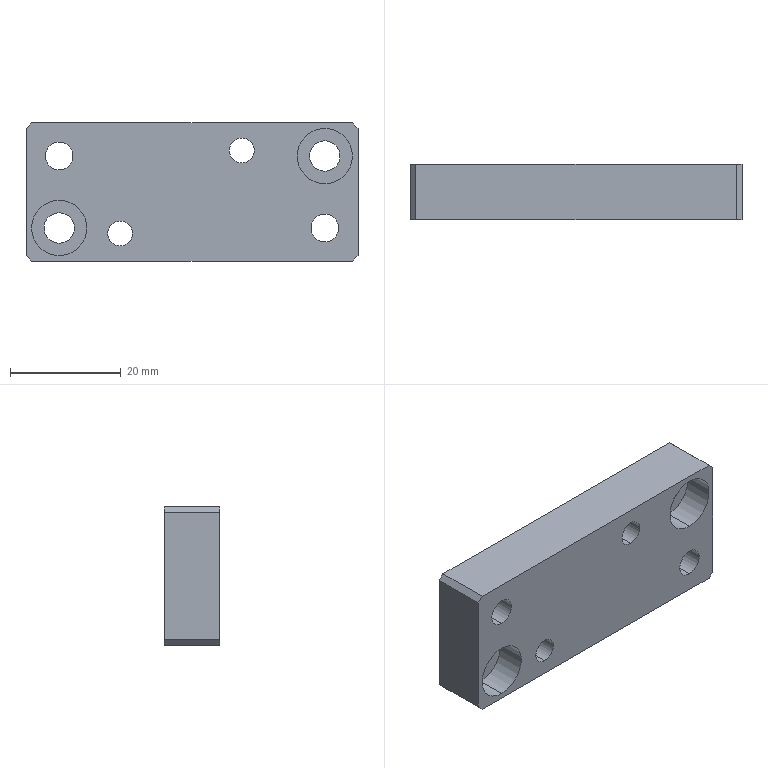Part | STEP file | PN_0033 | 1 solid | 34 faces | box 60 x 10 x 25 mm | volume 12893 mm3 | cylinder 20 | plane 14 | commonest cylinder face diameters 4.5 x4 5 x4 5.5 x4 8 x4 10 x4